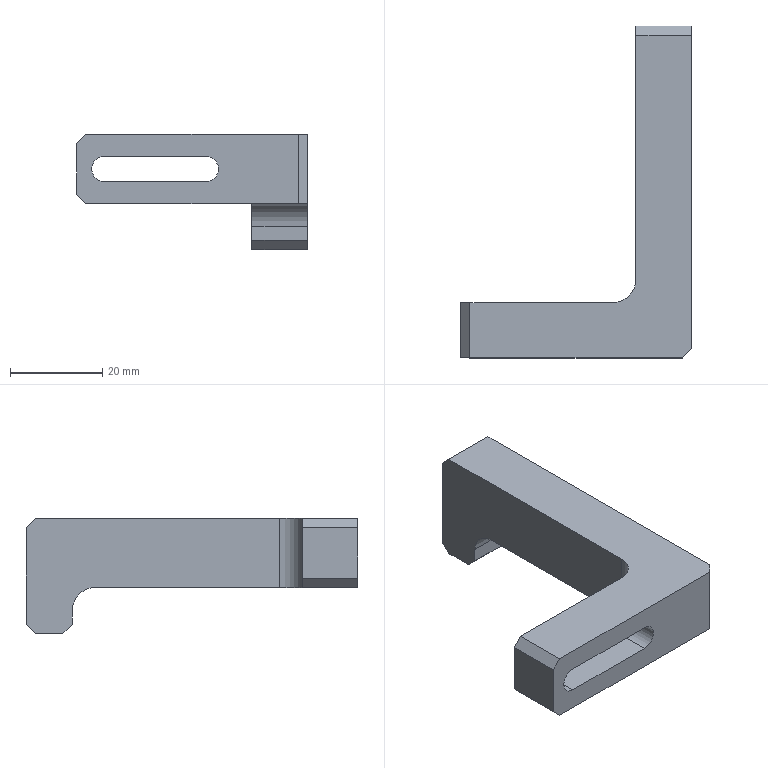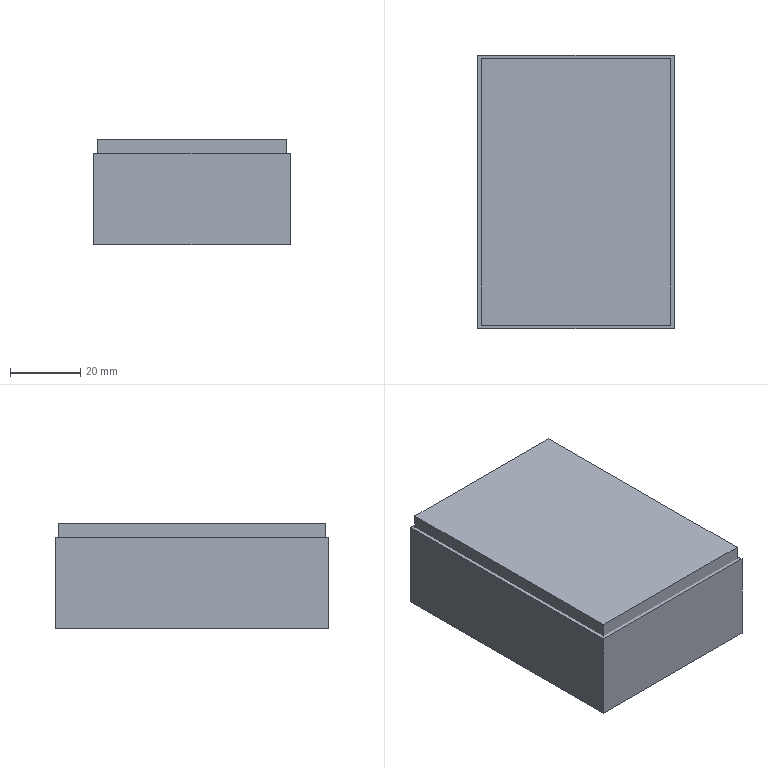CAM job | NX | 3+2 milling | part box 50 x 72 x 25 mm | stock box 56 x 78 x 30 mm
Tools:
number,name,description,diameter,corner_radius,flute_length,length,flutes
19,D80,Milling Tool-5 Parameters,80.0,0.0,50.0,75.0,2
15,D10,Milling Tool-5 Parameters,10.0,0.0,50.0,75.0,2
14,D10JING,Milling Tool-5 Parameters,10.0,0.0,50.0,75.0,2
1,D6A45,Milling Tool-5 Parameters,6.0,0.0,50.0,75.0,2
16,D4R0.5,Milling Tool-5 Parameters,4.0,0.5,50.0,75.0,2
16,D3,Milling Tool-5 Parameters,3.0,0.0,50.0,75.0,2
Operations:
program,operation,operation_type,tool,method,geometry_group,spindle_rpm,surface_speed,feed_per_tooth,feed_cut,feed_plunge,cut_length_mm,path_length_mm,cut_time_min,machine_time_min
1,FLOOR_WALL,VolumeBased25DMillingOperation,D80,METHOD,A,6500.0,1633.0,0.1154,1500.0,100.0,170.0,224.0,0.1133,0.1187
1,ADAPTIVE_MILLING,CavityMilling,D10,METHOD,A,9500.0,298.0,0.1842,3500.0,1000.0,11761.15,11865.15,3.362,3.373
1,ZLEVEL_PROFILE_COPY_1,ZLevelMilling,D10JING,METHOD,A,9500.0,298.0,0.0632,1200.0,1000.0,779.942,861.942,0.7343,0.7425
1,PLANAR_MILL_COPY_COPY_COPY,PlanarMilling,D6A45,METHOD,A,9500.0,179.0,0.0658,1250.0,100.0,251.432,310.432,0.2011,0.207
1,PLANAR_MILL_COPY_COPY_COPY_COPY,PlanarMilling,D6A45,METHOD,A,9500.0,179.0,0.0658,1250.0,100.0,34.189,229.395,0.0274,0.0469
2,PLANAR_MILL,PlanarMilling,D10,METHOD,B,9500.0,298.0,0.1053,2000.0,100.0,809.2,1434.469,0.4046,0.4671
2,FLOOR_WALL_COPY,VolumeBased25DMillingOperation,D80,METHOD,B,6500.0,1633.0,0.1154,1500.0,100.0,840.0,1738.001,0.56,0.6498
2,FLOOR_WALL_1,VolumeBased25DMillingOperation,D10,METHOD,B,9500.0,298.0,0.1316,2500.0,100.0,4215.68,4289.48,1.686,1.694
2,FLOOR_WALL_2,VolumeBased25DMillingOperation,D10JING,METHOD,B,9500.0,298.0,0.0789,1500.0,100.0,539.809,688.309,0.3599,0.3747
2,ZLEVEL_PROFILE,ZLevelMilling,D4R0.5,METHOD,B,9500.0,119.0,0.1316,2500.0,100.0,2189.661,2253.682,0.8759,0.8823
2,ZLEVEL_PROFILE_COPY,ZLevelMilling,D4R0.5,METHOD,B,9500.0,119.0,0.1316,2500.0,100.0,603.079,659.649,0.2412,0.2469
2,PLANAR_MILL_COPY_COPY_COPY_COPY_1,PlanarMilling,D6A45,METHOD,B,9500.0,179.0,0.0658,1250.0,100.0,197.012,276.012,0.1576,0.1655
2,PLANAR_MILL_COPY_COPY_COPY_COPY_1_COPY,PlanarMilling,D6A45,METHOD,B,9500.0,179.0,0.0658,1250.0,100.0,18.711,100.711,0.015,0.0232
3,ZLEVEL_PROFILE_COPY_COPY_1,ZLevelMilling,D3,METHOD,C,9500.0,89.0,0.0632,1200.0,1000.0,2555.499,2626.299,2.132,2.139
3,PLANAR_MILL_COPY_COPY_COPY_COPY_2,PlanarMilling,D6A45,METHOD,C,9500.0,179.0,0.0658,1250.0,100.0,62.335,121.335,0.0499,0.0558